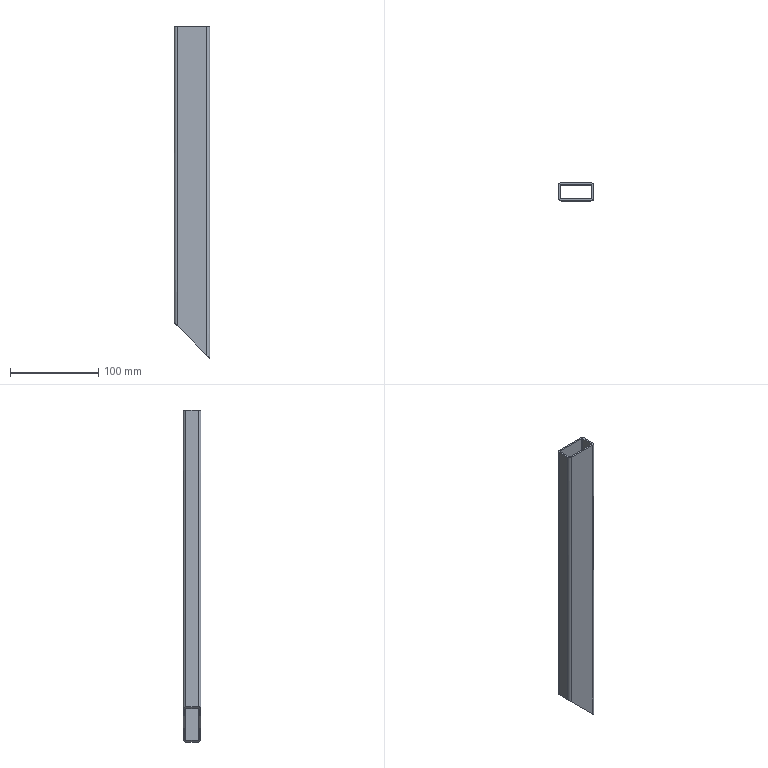Part | SolidWorks | features BaseBody 1 | 1 solid | 18 faces | box 40 x 20 x 377 mm | volume 77516 mm3 | plane 10 | cylinder 8 | commonest cylinder face diameters 2 x4 6 x4
STEP:
#1=CARTESIAN_POINT('',(18.,7.,-186.5));
#2=VERTEX_POINT('',#1);
#3=CARTESIAN_POINT('',(17.,8.,-185.5));
#4=VERTEX_POINT('',#3);
#5=CARTESIAN_POINT('',(18.,7.,-186.5));
#6=CARTESIAN_POINT('',(18.,7.586,-186.5));
#7=CARTESIAN_POINT('',(17.586,8.,-186.086));
#8=CARTESIAN_POINT('',(17.,8.,-185.5));
#9=(BOUNDED_CURVE()B_SPLINE_CURVE(3,(#5,#6,#7,#8),.UNSPECIFIED.,.F.,.F.)B_SPLINE_CURVE_WITH_KNOTS((4,4),(0.,1.571),.UNSPECIFIED.)CURVE()GEOMETRIC_REPRESENTATION_ITEM()RATIONAL_B_SPLINE_CURVE((1.,0.8047,0.8047,1.))REPRESENTATION_ITEM(''));
#10=EDGE_CURVE('',#2,#4,#9,.T.);
#11=ORIENTED_EDGE('',*,*,#10,.T.);
#12=CARTESIAN_POINT('',(-17.,8.,-151.5));
#13=VERTEX_POINT('',#12);
#14=CARTESIAN_POINT('',(-187.,8.,18.5));
#15=DIRECTION('',(-0.7071,0.,0.7071));
#16=VECTOR('',#15,1000.);
#17=LINE('',#14,#16);
#18=EDGE_CURVE('',#4,#13,#17,.T.);
#19=ORIENTED_EDGE('',*,*,#18,.T.);
#20=CARTESIAN_POINT('',(-18.,7.,-150.5));
#21=VERTEX_POINT('',#20);
#22=CARTESIAN_POINT('',(-17.,8.,-151.5));
#23=CARTESIAN_POINT('',(-17.586,8.,-150.914));
#24=CARTESIAN_POINT('',(-18.,7.586,-150.5));
#25=CARTESIAN_POINT('',(-18.,7.,-150.5));
#26=(BOUNDED_CURVE()B_SPLINE_CURVE(3,(#22,#23,#24,#25),.UNSPECIFIED.,.F.,.F.)B_SPLINE_CURVE_WITH_KNOTS((4,4),(1.571,3.142),.UNSPECIFIED.)CURVE()GEOMETRIC_REPRESENTATION_ITEM()RATIONAL_B_SPLINE_CURVE((1.,0.8047,0.8047,1.))REPRESENTATION_ITEM(''));
#27=EDGE_CURVE('',#13,#21,#26,.T.);
#28=ORIENTED_EDGE('',*,*,#27,.T.);
#29=CARTESIAN_POINT('',(-18.,-7.,-150.5));
#30=VERTEX_POINT('',#29);
#31=CARTESIAN_POINT('',(-18.,7.,-150.5));
#32=DIRECTION('',(0.,-1.,0.));
#33=VECTOR('',#32,1000.);
#34=LINE('',#31,#33);
#35=EDGE_CURVE('',#21,#30,#34,.T.);
#36=ORIENTED_EDGE('',*,*,#35,.T.);
#37=CARTESIAN_POINT('',(-17.,-8.,-151.5));
#38=VERTEX_POINT('',#37);
#39=CARTESIAN_POINT('',(-18.,-7.,-150.5));
#40=CARTESIAN_POINT('',(-18.,-7.586,-150.5));
#41=CARTESIAN_POINT('',(-17.586,-8.,-150.914));
#42=CARTESIAN_POINT('',(-17.,-8.,-151.5));
#43=(BOUNDED_CURVE()B_SPLINE_CURVE(3,(#39,#40,#41,#42),.UNSPECIFIED.,.F.,.F.)B_SPLINE_CURVE_WITH_KNOTS((4,4),(3.142,4.712),.UNSPECIFIED.)CURVE()GEOMETRIC_REPRESENTATION_ITEM()RATIONAL_B_SPLINE_CURVE((1.,0.8047,0.8047,1.))REPRESENTATION_ITEM(''));
#44=EDGE_CURVE('',#30,#38,#43,.T.);
#45=ORIENTED_EDGE('',*,*,#44,.T.);
#46=CARTESIAN_POINT('',(17.,-8.,-185.5));
#47=VERTEX_POINT('',#46);
#48=CARTESIAN_POINT('',(-187.,-8.,18.5));
#49=DIRECTION('',(0.7071,0.,-0.7071));
#50=VECTOR('',#49,1000.);
#51=LINE('',#48,#50);
#52=EDGE_CURVE('',#38,#47,#51,.T.);
#53=ORIENTED_EDGE('',*,*,#52,.T.);
#54=CARTESIAN_POINT('',(18.,-7.,-186.5));
#55=VERTEX_POINT('',#54);
#56=CARTESIAN_POINT('',(17.,-8.,-185.5));
#57=CARTESIAN_POINT('',(17.586,-8.,-186.086));
#58=CARTESIAN_POINT('',(18.,-7.586,-186.5));
#59=CARTESIAN_POINT('',(18.,-7.,-186.5));
#60=(BOUNDED_CURVE()B_SPLINE_CURVE(3,(#56,#57,#58,#59),.UNSPECIFIED.,.F.,.F.)B_SPLINE_CURVE_WITH_KNOTS((4,4),(4.712,6.283),.UNSPECIFIED.)CURVE()GEOMETRIC_REPRESENTATION_ITEM()RATIONAL_B_SPLINE_CURVE((1.,0.8047,0.8047,1.))REPRESENTATION_ITEM(''));
#61=EDGE_CURVE('',#47,#55,#60,.T.);
#62=ORIENTED_EDGE('',*,*,#61,.T.);
#63=CARTESIAN_POINT('',(18.,7.,-186.5));
#64=DIRECTION('',(0.,1.,0.));
#65=VECTOR('',#64,1000.);
#66=LINE('',#63,#65);
#67=EDGE_CURVE('',#55,#2,#66,.T.);
#68=ORIENTED_EDGE('',*,*,#67,.T.);
#69=EDGE_LOOP('',(#11,#19,#28,#36,#45,#53,#62,#68));
#70=FACE_BOUND('',#69,.T.);
#71=CARTESIAN_POINT('',(17.,-10.,-185.5));
#72=VERTEX_POINT('',#71);
#73=CARTESIAN_POINT('',(-17.,-10.,-151.5));
#74=VERTEX_POINT('',#73);
#75=CARTESIAN_POINT('',(-20.,-10.,-148.5));
#76=DIRECTION('',(-0.7071,0.,0.7071));
#77=VECTOR('',#76,1000.);
#78=LINE('',#75,#77);
#79=EDGE_CURVE('',#72,#74,#78,.T.);
#80=ORIENTED_EDGE('',*,*,#79,.T.);
#81=CARTESIAN_POINT('',(-20.,-7.,-148.5));
#82=VERTEX_POINT('',#81);
#83=CARTESIAN_POINT('',(-20.,-7.,-148.5));
#84=CARTESIAN_POINT('',(-20.,-8.757,-148.5));
#85=CARTESIAN_POINT('',(-18.757,-10.,-149.743));
#86=CARTESIAN_POINT('',(-17.,-10.,-151.5));
#87=(BOUNDED_CURVE()B_SPLINE_CURVE(3,(#83,#84,#85,#86),.UNSPECIFIED.,.F.,.T.)B_SPLINE_CURVE_WITH_KNOTS((4,4),(3.142,4.712),.UNSPECIFIED.)CURVE()GEOMETRIC_REPRESENTATION_ITEM()RATIONAL_B_SPLINE_CURVE((1.,0.8047,0.8047,1.))REPRESENTATION_ITEM(''));
#88=EDGE_CURVE('',#82,#74,#87,.T.);
#89=ORIENTED_EDGE('',*,*,#88,.F.);
#90=CARTESIAN_POINT('',(-20.,7.,-148.5));
#91=VERTEX_POINT('',#90);
#92=CARTESIAN_POINT('',(-20.,10.,-148.5));
#93=DIRECTION('',(0.,-1.,0.));
#94=VECTOR('',#93,1000.);
#95=LINE('',#92,#94);
#96=EDGE_CURVE('',#91,#82,#95,.T.);
#97=ORIENTED_EDGE('',*,*,#96,.F.);
#98=CARTESIAN_POINT('',(-17.,10.,-151.5));
#99=VERTEX_POINT('',#98);
#100=CARTESIAN_POINT('',(-17.,10.,-151.5));
#101=CARTESIAN_POINT('',(-18.757,10.,-149.743));
#102=CARTESIAN_POINT('',(-20.,8.757,-148.5));
#103=CARTESIAN_POINT('',(-20.,7.,-148.5));
#104=(BOUNDED_CURVE()B_SPLINE_CURVE(3,(#100,#101,#102,#103),.UNSPECIFIED.,.F.,.F.)B_SPLINE_CURVE_WITH_KNOTS((4,4),(1.571,3.142),.UNSPECIFIED.)CURVE()GEOMETRIC_REPRESENTATION_ITEM()RATIONAL_B_SPLINE_CURVE((1.,0.8047,0.8047,1.))REPRESENTATION_ITEM(''));
#105=EDGE_CURVE('',#99,#91,#104,.T.);
#106=ORIENTED_EDGE('',*,*,#105,.F.);
#107=CARTESIAN_POINT('',(17.,10.,-185.5));
#108=VERTEX_POINT('',#107);
#109=CARTESIAN_POINT('',(-20.,10.,-148.5));
#110=DIRECTION('',(-0.7071,0.,0.7071));
#111=VECTOR('',#110,1000.);
#112=LINE('',#109,#111);
#113=EDGE_CURVE('',#108,#99,#112,.T.);
#114=ORIENTED_EDGE('',*,*,#113,.F.);
#115=CARTESIAN_POINT('',(20.,7.,-188.5));
#116=VERTEX_POINT('',#115);
#117=CARTESIAN_POINT('',(20.,7.,-188.5));
#118=CARTESIAN_POINT('',(20.,8.757,-188.5));
#119=CARTESIAN_POINT('',(18.757,10.,-187.257));
#120=CARTESIAN_POINT('',(17.,10.,-185.5));
#121=(BOUNDED_CURVE()B_SPLINE_CURVE(3,(#117,#118,#119,#120),.UNSPECIFIED.,.F.,.F.)B_SPLINE_CURVE_WITH_KNOTS((4,4),(0.,1.571),.UNSPECIFIED.)CURVE()GEOMETRIC_REPRESENTATION_ITEM()RATIONAL_B_SPLINE_CURVE((1.,0.8047,0.8047,1.))REPRESENTATION_ITEM(''));
#122=EDGE_CURVE('',#116,#108,#121,.T.);
#123=ORIENTED_EDGE('',*,*,#122,.F.);
#124=CARTESIAN_POINT('',(20.,-7.,-188.5));
#125=VERTEX_POINT('',#124);
#126=CARTESIAN_POINT('',(20.,7.,-188.5));
#127=DIRECTION('',(0.,1.,0.));
#128=VECTOR('',#127,1000.);
#129=LINE('',#126,#128);
#130=EDGE_CURVE('',#125,#116,#129,.T.);
#131=ORIENTED_EDGE('',*,*,#130,.F.);
#132=CARTESIAN_POINT('',(17.,-10.,-185.5));
#133=CARTESIAN_POINT('',(18.757,-10.,-187.257));
#134=CARTESIAN_POINT('',(20.,-8.757,-188.5));
#135=CARTESIAN_POINT('',(20.,-7.,-188.5));
#136=(BOUNDED_CURVE()B_SPLINE_CURVE(3,(#132,#133,#134,#135),.UNSPECIFIED.,.F.,.T.)B_SPLINE_CURVE_WITH_KNOTS((4,4),(4.712,6.283),.UNSPECIFIED.)CURVE()GEOMETRIC_REPRESENTATION_ITEM()RATIONAL_B_SPLINE_CURVE((1.,0.8047,0.8047,1.))REPRESENTATION_ITEM(''));
#137=EDGE_CURVE('',#72,#125,#136,.T.);
#138=ORIENTED_EDGE('',*,*,#137,.F.);
#139=EDGE_LOOP('',(#80,#89,#97,#106,#114,#123,#131,#138));
#140=FACE_OUTER_BOUND('',#139,.T.);
#141=CARTESIAN_POINT('',(-20.,10.,-148.5));
#142=DIRECTION('',(0.7071,0.,0.7071));
#143=DIRECTION('',(0.,-1.,0.));
#144=AXIS2_PLACEMENT_3D('',#141,#142,#143);
#145=PLANE('',#144);
#146=ADVANCED_FACE('',(#70,#140),#145,.F.);
#147=ORIENTED_EDGE('',*,*,#67,.F.);
#148=CARTESIAN_POINT('',(18.,-7.,188.5));
#149=VERTEX_POINT('',#148);
#150=CARTESIAN_POINT('',(18.,-7.,188.5));
#151=DIRECTION('',(0.,0.,-1.));
#152=VECTOR('',#151,1000.);
#153=LINE('',#150,#152);
#154=EDGE_CURVE('',#149,#55,#153,.T.);
#155=ORIENTED_EDGE('',*,*,#154,.F.);
#156=CARTESIAN_POINT('',(18.,7.,188.5));
#157=VERTEX_POINT('',#156);
#158=CARTESIAN_POINT('',(18.,7.,188.5));
#159=DIRECTION('',(0.,1.,0.));
#160=VECTOR('',#159,1000.);
#161=LINE('',#158,#160);
#162=EDGE_CURVE('',#149,#157,#161,.T.);
#163=ORIENTED_EDGE('',*,*,#162,.T.);
#164=CARTESIAN_POINT('',(18.,7.,188.5));
#165=DIRECTION('',(0.,0.,-1.));
#166=VECTOR('',#165,1000.);
#167=LINE('',#164,#166);
#168=EDGE_CURVE('',#157,#2,#167,.T.);
#169=ORIENTED_EDGE('',*,*,#168,.T.);
#170=EDGE_LOOP('',(#147,#155,#163,#169));
#171=FACE_OUTER_BOUND('',#170,.T.);
#172=CARTESIAN_POINT('',(18.,7.,188.5));
#173=DIRECTION('',(-1.,0.,0.));
#174=DIRECTION('',(0.,0.,1.));
#175=AXIS2_PLACEMENT_3D('',#172,#173,#174);
#176=PLANE('',#175);
#177=ADVANCED_FACE('',(#171),#176,.T.);
#178=ORIENTED_EDGE('',*,*,#61,.F.);
#179=CARTESIAN_POINT('',(17.,-8.,188.5));
#180=VERTEX_POINT('',#179);
#181=CARTESIAN_POINT('',(17.,-8.,188.5));
#182=DIRECTION('',(0.,0.,-1.));
#183=VECTOR('',#182,1000.);
#184=LINE('',#181,#183);
#185=EDGE_CURVE('',#180,#47,#184,.T.);
#186=ORIENTED_EDGE('',*,*,#185,.F.);
#187=CARTESIAN_POINT('',(17.,-7.,188.5));
#188=DIRECTION('',(0.,0.,1.));
#189=DIRECTION('',(1.,0.,0.));
#190=AXIS2_PLACEMENT_3D('',#187,#188,#189);
#191=CIRCLE('',#190,1.);
#192=EDGE_CURVE('',#180,#149,#191,.T.);
#193=ORIENTED_EDGE('',*,*,#192,.T.);
#194=ORIENTED_EDGE('',*,*,#154,.T.);
#195=EDGE_LOOP('',(#178,#186,#193,#194));
#196=FACE_OUTER_BOUND('',#195,.T.);
#197=CARTESIAN_POINT('',(17.,-7.,188.5));
#198=DIRECTION('',(0.,0.,-1.));
#199=DIRECTION('',(-1.,0.,0.));
#200=AXIS2_PLACEMENT_3D('',#197,#198,#199);
#201=CYLINDRICAL_SURFACE('',#200,1.);
#202=ADVANCED_FACE('',(#196),#201,.F.);
#203=ORIENTED_EDGE('',*,*,#52,.F.);
#204=CARTESIAN_POINT('',(-17.,-8.,188.5));
#205=VERTEX_POINT('',#204);
#206=CARTESIAN_POINT('',(-17.,-8.,188.5));
#207=DIRECTION('',(0.,0.,-1.));
#208=VECTOR('',#207,1000.);
#209=LINE('',#206,#208);
#210=EDGE_CURVE('',#205,#38,#209,.T.);
#211=ORIENTED_EDGE('',*,*,#210,.F.);
#212=CARTESIAN_POINT('',(-17.,-8.,188.5));
#213=DIRECTION('',(1.,0.,0.));
#214=VECTOR('',#213,1000.);
#215=LINE('',#212,#214);
#216=EDGE_CURVE('',#205,#180,#215,.T.);
#217=ORIENTED_EDGE('',*,*,#216,.T.);
#218=ORIENTED_EDGE('',*,*,#185,.T.);
#219=EDGE_LOOP('',(#203,#211,#217,#218));
#220=FACE_OUTER_BOUND('',#219,.T.);
#221=CARTESIAN_POINT('',(-17.,-8.,188.5));
#222=DIRECTION('',(0.,1.,0.));
#223=DIRECTION('',(1.,0.,0.));
#224=AXIS2_PLACEMENT_3D('',#221,#222,#223);
#225=PLANE('',#224);
#226=ADVANCED_FACE('',(#220),#225,.T.);
#227=ORIENTED_EDGE('',*,*,#44,.F.);
#228=CARTESIAN_POINT('',(-18.,-7.,188.5));
#229=VERTEX_POINT('',#228);
#230=CARTESIAN_POINT('',(-18.,-7.,188.5));
#231=DIRECTION('',(0.,0.,-1.));
#232=VECTOR('',#231,1000.);
#233=LINE('',#230,#232);
#234=EDGE_CURVE('',#229,#30,#233,.T.);
#235=ORIENTED_EDGE('',*,*,#234,.F.);
#236=CARTESIAN_POINT('',(-17.,-7.,188.5));
#237=DIRECTION('',(0.,0.,1.));
#238=DIRECTION('',(1.,0.,0.));
#239=AXIS2_PLACEMENT_3D('',#236,#237,#238);
#240=CIRCLE('',#239,1.);
#241=EDGE_CURVE('',#229,#205,#240,.T.);
#242=ORIENTED_EDGE('',*,*,#241,.T.);
#243=ORIENTED_EDGE('',*,*,#210,.T.);
#244=EDGE_LOOP('',(#227,#235,#242,#243));
#245=FACE_OUTER_BOUND('',#244,.T.);
#246=CARTESIAN_POINT('',(-17.,-7.,188.5));
#247=DIRECTION('',(0.,0.,-1.));
#248=DIRECTION('',(-1.,0.,0.));
#249=AXIS2_PLACEMENT_3D('',#246,#247,#248);
#250=CYLINDRICAL_SURFACE('',#249,1.);
#251=ADVANCED_FACE('',(#245),#250,.F.);
#252=ORIENTED_EDGE('',*,*,#35,.F.);
#253=CARTESIAN_POINT('',(-18.,7.,188.5));
#254=VERTEX_POINT('',#253);
#255=CARTESIAN_POINT('',(-18.,7.,188.5));
#256=DIRECTION('',(0.,0.,-1.));
#257=VECTOR('',#256,1000.);
#258=LINE('',#255,#257);
#259=EDGE_CURVE('',#254,#21,#258,.T.);
#260=ORIENTED_EDGE('',*,*,#259,.F.);
#261=CARTESIAN_POINT('',(-18.,7.,188.5));
#262=DIRECTION('',(0.,-1.,0.));
#263=VECTOR('',#262,1000.);
#264=LINE('',#261,#263);
#265=EDGE_CURVE('',#254,#229,#264,.T.);
#266=ORIENTED_EDGE('',*,*,#265,.T.);
#267=ORIENTED_EDGE('',*,*,#234,.T.);
#268=EDGE_LOOP('',(#252,#260,#266,#267));
#269=FACE_OUTER_BOUND('',#268,.T.);
#270=CARTESIAN_POINT('',(-18.,7.,188.5));
#271=DIRECTION('',(1.,0.,0.));
#272=DIRECTION('',(0.,-1.,0.));
#273=AXIS2_PLACEMENT_3D('',#270,#271,#272);
#274=PLANE('',#273);
#275=ADVANCED_FACE('',(#269),#274,.T.);
#276=ORIENTED_EDGE('',*,*,#27,.F.);
#277=CARTESIAN_POINT('',(-17.,8.,188.5));
#278=VERTEX_POINT('',#277);
#279=CARTESIAN_POINT('',(-17.,8.,188.5));
#280=DIRECTION('',(0.,0.,-1.));
#281=VECTOR('',#280,1000.);
#282=LINE('',#279,#281);
#283=EDGE_CURVE('',#278,#13,#282,.T.);
#284=ORIENTED_EDGE('',*,*,#283,.F.);
#285=CARTESIAN_POINT('',(-17.,7.,188.5));
#286=DIRECTION('',(0.,0.,1.));
#287=DIRECTION('',(1.,0.,0.));
#288=AXIS2_PLACEMENT_3D('',#285,#286,#287);
#289=CIRCLE('',#288,1.);
#290=EDGE_CURVE('',#278,#254,#289,.T.);
#291=ORIENTED_EDGE('',*,*,#290,.T.);
#292=ORIENTED_EDGE('',*,*,#259,.T.);
#293=EDGE_LOOP('',(#276,#284,#291,#292));
#294=FACE_OUTER_BOUND('',#293,.T.);
#295=CARTESIAN_POINT('',(-17.,7.,188.5));
#296=DIRECTION('',(0.,0.,-1.));
#297=DIRECTION('',(-1.,0.,0.));
#298=AXIS2_PLACEMENT_3D('',#295,#296,#297);
#299=CYLINDRICAL_SURFACE('',#298,1.);
#300=ADVANCED_FACE('',(#294),#299,.F.);
#301=ORIENTED_EDGE('',*,*,#18,.F.);
#302=CARTESIAN_POINT('',(17.,8.,188.5));
#303=VERTEX_POINT('',#302);
#304=CARTESIAN_POINT('',(17.,8.,188.5));
#305=DIRECTION('',(0.,0.,-1.));
#306=VECTOR('',#305,1000.);
#307=LINE('',#304,#306);
#308=EDGE_CURVE('',#303,#4,#307,.T.);
#309=ORIENTED_EDGE('',*,*,#308,.F.);
#310=CARTESIAN_POINT('',(-17.,8.,188.5));
#311=DIRECTION('',(-1.,0.,0.));
#312=VECTOR('',#311,1000.);
#313=LINE('',#310,#312);
#314=EDGE_CURVE('',#303,#278,#313,.T.);
#315=ORIENTED_EDGE('',*,*,#314,.T.);
#316=ORIENTED_EDGE('',*,*,#283,.T.);
#317=EDGE_LOOP('',(#301,#309,#315,#316));
#318=FACE_OUTER_BOUND('',#317,.T.);
#319=CARTESIAN_POINT('',(-17.,8.,188.5));
#320=DIRECTION('',(0.,-1.,0.));
#321=DIRECTION('',(0.,0.,-1.));
#322=AXIS2_PLACEMENT_3D('',#319,#320,#321);
#323=PLANE('',#322);
#324=ADVANCED_FACE('',(#318),#323,.T.);
#325=ORIENTED_EDGE('',*,*,#10,.F.);
#326=ORIENTED_EDGE('',*,*,#168,.F.);
#327=CARTESIAN_POINT('',(17.,7.,188.5));
#328=DIRECTION('',(0.,0.,1.));
#329=DIRECTION('',(-1.,0.,0.));
#330=AXIS2_PLACEMENT_3D('',#327,#328,#329);
#331=CIRCLE('',#330,1.);
#332=EDGE_CURVE('',#157,#303,#331,.T.);
#333=ORIENTED_EDGE('',*,*,#332,.T.);
#334=ORIENTED_EDGE('',*,*,#308,.T.);
#335=EDGE_LOOP('',(#325,#326,#333,#334));
#336=FACE_OUTER_BOUND('',#335,.T.);
#337=CARTESIAN_POINT('',(17.,7.,188.5));
#338=DIRECTION('',(0.,0.,-1.));
#339=DIRECTION('',(-1.,0.,0.));
#340=AXIS2_PLACEMENT_3D('',#337,#338,#339);
#341=CYLINDRICAL_SURFACE('',#340,1.);
#342=ADVANCED_FACE('',(#336),#341,.F.);
#343=CARTESIAN_POINT('',(-17.,-10.,188.5));
#344=VERTEX_POINT('',#343);
#345=CARTESIAN_POINT('',(-17.,-10.,188.5));
#346=DIRECTION('',(0.,0.,-1.));
#347=VECTOR('',#346,1000.);
#348=LINE('',#345,#347);
#349=EDGE_CURVE('',#344,#74,#348,.T.);
#350=ORIENTED_EDGE('',*,*,#349,.T.);
#351=ORIENTED_EDGE('',*,*,#79,.F.);
#352=CARTESIAN_POINT('',(17.,-10.,188.5));
#353=VERTEX_POINT('',#352);
#354=CARTESIAN_POINT('',(17.,-10.,188.5));
#355=DIRECTION('',(0.,0.,-1.));
#356=VECTOR('',#355,1000.);
#357=LINE('',#354,#356);
#358=EDGE_CURVE('',#353,#72,#357,.T.);
#359=ORIENTED_EDGE('',*,*,#358,.F.);
#360=CARTESIAN_POINT('',(-17.,-10.,188.5));
#361=DIRECTION('',(1.,0.,0.));
#362=VECTOR('',#361,1000.);
#363=LINE('',#360,#362);
#364=EDGE_CURVE('',#344,#353,#363,.T.);
#365=ORIENTED_EDGE('',*,*,#364,.F.);
#366=EDGE_LOOP('',(#350,#351,#359,#365));
#367=FACE_OUTER_BOUND('',#366,.T.);
#368=CARTESIAN_POINT('',(-17.,-10.,188.5));
#369=DIRECTION('',(0.,1.,0.));
#370=DIRECTION('',(1.,0.,0.));
#371=AXIS2_PLACEMENT_3D('',#368,#369,#370);
#372=PLANE('',#371);
#373=ADVANCED_FACE('',(#367),#372,.F.);
#374=CARTESIAN_POINT('',(-20.,-7.,188.5));
#375=VERTEX_POINT('',#374);
#376=CARTESIAN_POINT('',(-20.,-7.,188.5));
#377=DIRECTION('',(0.,0.,-1.));
#378=VECTOR('',#377,1000.);
#379=LINE('',#376,#378);
#380=EDGE_CURVE('',#375,#82,#379,.T.);
#381=ORIENTED_EDGE('',*,*,#380,.T.);
#382=ORIENTED_EDGE('',*,*,#88,.T.);
#383=ORIENTED_EDGE('',*,*,#349,.F.);
#384=CARTESIAN_POINT('',(-17.,-7.,188.5));
#385=DIRECTION('',(0.,0.,1.));
#386=DIRECTION('',(1.,0.,0.));
#387=AXIS2_PLACEMENT_3D('',#384,#385,#386);
#388=CIRCLE('',#387,3.);
#389=EDGE_CURVE('',#375,#344,#388,.T.);
#390=ORIENTED_EDGE('',*,*,#389,.F.);
#391=EDGE_LOOP('',(#381,#382,#383,#390));
#392=FACE_OUTER_BOUND('',#391,.T.);
#393=CARTESIAN_POINT('',(-17.,-7.,188.5));
#394=DIRECTION('',(0.,0.,-1.));
#395=DIRECTION('',(-1.,0.,0.));
#396=AXIS2_PLACEMENT_3D('',#393,#394,#395);
#397=CYLINDRICAL_SURFACE('',#396,3.);
#398=ADVANCED_FACE('',(#392),#397,.T.);
#399=CARTESIAN_POINT('',(-20.,7.,188.5));
#400=VERTEX_POINT('',#399);
#401=CARTESIAN_POINT('',(-20.,7.,188.5));
#402=DIRECTION('',(0.,0.,-1.));
#403=VECTOR('',#402,1000.);
#404=LINE('',#401,#403);
#405=EDGE_CURVE('',#400,#91,#404,.T.);
#406=ORIENTED_EDGE('',*,*,#405,.T.);
#407=ORIENTED_EDGE('',*,*,#96,.T.);
#408=ORIENTED_EDGE('',*,*,#380,.F.);
#409=CARTESIAN_POINT('',(-20.,7.,188.5));
#410=DIRECTION('',(0.,-1.,0.));
#411=VECTOR('',#410,1000.);
#412=LINE('',#409,#411);
#413=EDGE_CURVE('',#400,#375,#412,.T.);
#414=ORIENTED_EDGE('',*,*,#413,.F.);
#415=EDGE_LOOP('',(#406,#407,#408,#414));
#416=FACE_OUTER_BOUND('',#415,.T.);
#417=CARTESIAN_POINT('',(-20.,7.,188.5));
#418=DIRECTION('',(1.,0.,0.));
#419=DIRECTION('',(0.,1.,0.));
#420=AXIS2_PLACEMENT_3D('',#417,#418,#419);
#421=PLANE('',#420);
#422=ADVANCED_FACE('',(#416),#421,.F.);
#423=CARTESIAN_POINT('',(-17.,10.,188.5));
#424=VERTEX_POINT('',#423);
#425=CARTESIAN_POINT('',(-17.,10.,188.5));
#426=DIRECTION('',(0.,0.,-1.));
#427=VECTOR('',#426,1000.);
#428=LINE('',#425,#427);
#429=EDGE_CURVE('',#424,#99,#428,.T.);
#430=ORIENTED_EDGE('',*,*,#429,.T.);
#431=ORIENTED_EDGE('',*,*,#105,.T.);
#432=ORIENTED_EDGE('',*,*,#405,.F.);
#433=CARTESIAN_POINT('',(-17.,7.,188.5));
#434=DIRECTION('',(0.,0.,1.));
#435=DIRECTION('',(1.,0.,0.));
#436=AXIS2_PLACEMENT_3D('',#433,#434,#435);
#437=CIRCLE('',#436,3.);
#438=EDGE_CURVE('',#424,#400,#437,.T.);
#439=ORIENTED_EDGE('',*,*,#438,.F.);
#440=EDGE_LOOP('',(#430,#431,#432,#439));
#441=FACE_OUTER_BOUND('',#440,.T.);
#442=CARTESIAN_POINT('',(-17.,7.,188.5));
#443=DIRECTION('',(0.,0.,-1.));
#444=DIRECTION('',(-1.,0.,0.));
#445=AXIS2_PLACEMENT_3D('',#442,#443,#444);
#446=CYLINDRICAL_SURFACE('',#445,3.);
#447=ADVANCED_FACE('',(#441),#446,.T.);
#448=CARTESIAN_POINT('',(17.,10.,188.5));
#449=VERTEX_POINT('',#448);
#450=CARTESIAN_POINT('',(17.,10.,188.5));
#451=DIRECTION('',(0.,0.,-1.));
#452=VECTOR('',#451,1000.);
#453=LINE('',#450,#452);
#454=EDGE_CURVE('',#449,#108,#453,.T.);
#455=ORIENTED_EDGE('',*,*,#454,.T.);
#456=ORIENTED_EDGE('',*,*,#113,.T.);
#457=ORIENTED_EDGE('',*,*,#429,.F.);
#458=CARTESIAN_POINT('',(-17.,10.,188.5));
#459=DIRECTION('',(-1.,0.,0.));
#460=VECTOR('',#459,1000.);
#461=LINE('',#458,#460);
#462=EDGE_CURVE('',#449,#424,#461,.T.);
#463=ORIENTED_EDGE('',*,*,#462,.F.);
#464=EDGE_LOOP('',(#455,#456,#457,#463));
#465=FACE_OUTER_BOUND('',#464,.T.);
#466=CARTESIAN_POINT('',(-17.,10.,188.5));
#467=DIRECTION('',(0.,-1.,0.));
#468=DIRECTION('',(0.,0.,-1.));
#469=AXIS2_PLACEMENT_3D('',#466,#467,#468);
#470=PLANE('',#469);
#471=ADVANCED_FACE('',(#465),#470,.F.);
#472=CARTESIAN_POINT('',(20.,7.,188.5));
#473=VERTEX_POINT('',#472);
#474=CARTESIAN_POINT('',(20.,7.,188.5));
#475=DIRECTION('',(0.,0.,-1.));
#476=VECTOR('',#475,1000.);
#477=LINE('',#474,#476);
#478=EDGE_CURVE('',#473,#116,#477,.T.);
#479=ORIENTED_EDGE('',*,*,#478,.T.);
#480=ORIENTED_EDGE('',*,*,#122,.T.);
#481=ORIENTED_EDGE('',*,*,#454,.F.);
#482=CARTESIAN_POINT('',(17.,7.,188.5));
#483=DIRECTION('',(0.,0.,1.));
#484=DIRECTION('',(-1.,0.,0.));
#485=AXIS2_PLACEMENT_3D('',#482,#483,#484);
#486=CIRCLE('',#485,3.);
#487=EDGE_CURVE('',#473,#449,#486,.T.);
#488=ORIENTED_EDGE('',*,*,#487,.F.);
#489=EDGE_LOOP('',(#479,#480,#481,#488));
#490=FACE_OUTER_BOUND('',#489,.T.);
#491=CARTESIAN_POINT('',(17.,7.,188.5));
#492=DIRECTION('',(0.,0.,-1.));
#493=DIRECTION('',(-1.,0.,0.));
#494=AXIS2_PLACEMENT_3D('',#491,#492,#493);
#495=CYLINDRICAL_SURFACE('',#494,3.);
#496=ADVANCED_FACE('',(#490),#495,.T.);
#497=ORIENTED_EDGE('',*,*,#130,.T.);
#498=ORIENTED_EDGE('',*,*,#478,.F.);
#499=CARTESIAN_POINT('',(20.,-7.,188.5));
#500=VERTEX_POINT('',#499);
#501=CARTESIAN_POINT('',(20.,7.,188.5));
#502=DIRECTION('',(0.,1.,0.));
#503=VECTOR('',#502,1000.);
#504=LINE('',#501,#503);
#505=EDGE_CURVE('',#500,#473,#504,.T.);
#506=ORIENTED_EDGE('',*,*,#505,.F.);
#507=CARTESIAN_POINT('',(20.,-7.,188.5));
#508=DIRECTION('',(0.,0.,-1.));
#509=VECTOR('',#508,1000.);
#510=LINE('',#507,#509);
#511=EDGE_CURVE('',#500,#125,#510,.T.);
#512=ORIENTED_EDGE('',*,*,#511,.T.);
#513=EDGE_LOOP('',(#497,#498,#506,#512));
#514=FACE_OUTER_BOUND('',#513,.T.);
#515=CARTESIAN_POINT('',(20.,7.,188.5));
#516=DIRECTION('',(-1.,0.,0.));
#517=DIRECTION('',(0.,0.,1.));
#518=AXIS2_PLACEMENT_3D('',#515,#516,#517);
#519=PLANE('',#518);
#520=ADVANCED_FACE('',(#514),#519,.F.);
#521=ORIENTED_EDGE('',*,*,#358,.T.);
#522=ORIENTED_EDGE('',*,*,#137,.T.);
#523=ORIENTED_EDGE('',*,*,#511,.F.);
#524=CARTESIAN_POINT('',(17.,-7.,188.5));
#525=DIRECTION('',(0.,0.,1.));
#526=DIRECTION('',(1.,0.,0.));
#527=AXIS2_PLACEMENT_3D('',#524,#525,#526);
#528=CIRCLE('',#527,3.);
#529=EDGE_CURVE('',#353,#500,#528,.T.);
#530=ORIENTED_EDGE('',*,*,#529,.F.);
#531=EDGE_LOOP('',(#521,#522,#523,#530));
#532=FACE_OUTER_BOUND('',#531,.T.);
#533=CARTESIAN_POINT('',(17.,-7.,188.5));
#534=DIRECTION('',(0.,0.,-1.));
#535=DIRECTION('',(-1.,0.,0.));
#536=AXIS2_PLACEMENT_3D('',#533,#534,#535);
#537=CYLINDRICAL_SURFACE('',#536,3.);
#538=ADVANCED_FACE('',(#532),#537,.T.);
#539=ORIENTED_EDGE('',*,*,#314,.F.);
#540=ORIENTED_EDGE('',*,*,#332,.F.);
#541=ORIENTED_EDGE('',*,*,#162,.F.);
#542=ORIENTED_EDGE('',*,*,#192,.F.);
#543=ORIENTED_EDGE('',*,*,#216,.F.);
#544=ORIENTED_EDGE('',*,*,#241,.F.);
#545=ORIENTED_EDGE('',*,*,#265,.F.);
#546=ORIENTED_EDGE('',*,*,#290,.F.);
#547=EDGE_LOOP('',(#539,#540,#541,#542,#543,#544,#545,#546));
#548=FACE_BOUND('',#547,.T.);
#549=ORIENTED_EDGE('',*,*,#529,.T.);
#550=ORIENTED_EDGE('',*,*,#505,.T.);
#551=ORIENTED_EDGE('',*,*,#487,.T.);
#552=ORIENTED_EDGE('',*,*,#462,.T.);
#553=ORIENTED_EDGE('',*,*,#438,.T.);
#554=ORIENTED_EDGE('',*,*,#413,.T.);
#555=ORIENTED_EDGE('',*,*,#389,.T.);
#556=ORIENTED_EDGE('',*,*,#364,.T.);
#557=EDGE_LOOP('',(#549,#550,#551,#552,#553,#554,#555,#556));
#558=FACE_OUTER_BOUND('',#557,.T.);
#559=CARTESIAN_POINT('',(17.,-7.,188.5));
#560=DIRECTION('',(0.,0.,1.));
#561=DIRECTION('',(1.,0.,0.));
#562=AXIS2_PLACEMENT_3D('',#559,#560,#561);
#563=PLANE('',#562);
#564=ADVANCED_FACE('',(#548,#558),#563,.T.);
#565=CLOSED_SHELL('',(#146,#177,#202,#226,#251,#275,#300,#324,#342,#373,#398,#422,#447,#471,#496,#520,#538,#564));
#566=MANIFOLD_SOLID_BREP('',#565);
#567=CARTESIAN_POINT('',(0.,0.,0.));
#568=DIRECTION('',(0.,0.,1.));
#569=DIRECTION('',(1.,0.,0.));
#570=AXIS2_PLACEMENT_3D('',#567,#568,#569);
#571=(LENGTH_UNIT()NAMED_UNIT(*)SI_UNIT(.MILLI.,.METRE.));
#572=UNCERTAINTY_MEASURE_WITH_UNIT(LENGTH_MEASURE(0.00001),#571,'','');
#573=(NAMED_UNIT(*)PLANE_ANGLE_UNIT()SI_UNIT($,.RADIAN.));
#574=(NAMED_UNIT(*)SI_UNIT($,.STERADIAN.)SOLID_ANGLE_UNIT());
#575=(GEOMETRIC_REPRESENTATION_CONTEXT(3)GLOBAL_UNCERTAINTY_ASSIGNED_CONTEXT((#572))GLOBAL_UNIT_ASSIGNED_CONTEXT((#571,#573,#574))REPRESENTATION_CONTEXT('',''));
#576=ADVANCED_BREP_SHAPE_REPRESENTATION('',(#566,#570),#575);